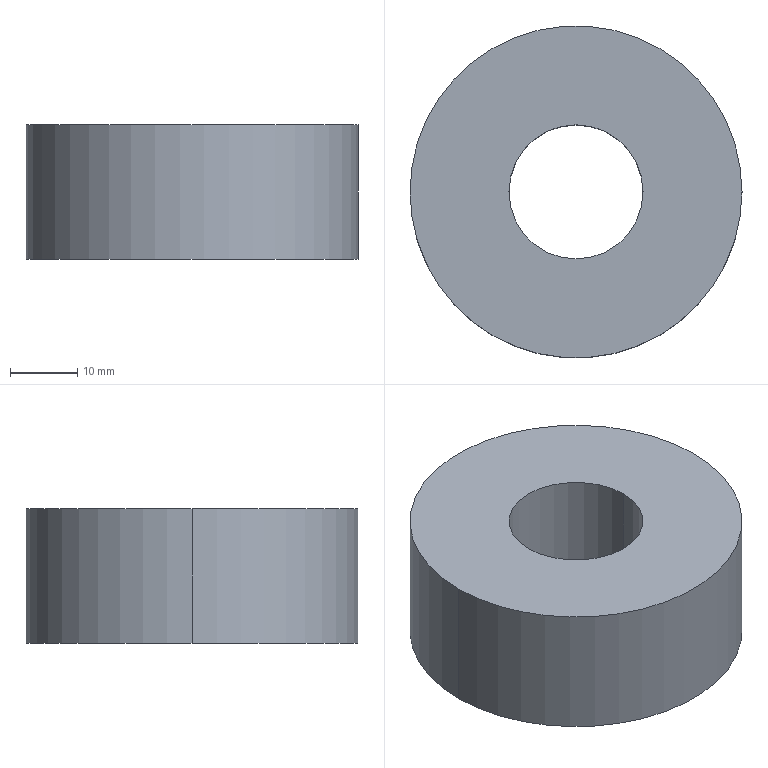Part | SolidWorks | features BaseBody 1 | 1 solid | 6 faces | box 49.497 x 49.497 x 20 mm | volume 32201 mm3 | cylinder 4 | plane 2 | commonest cylinder face diameters 20 x2 49.497 x2
STEP:
#1=CARTESIAN_POINT('',(2518.111,1500.936,20.));
#2=VERTEX_POINT('',#1);
#3=CARTESIAN_POINT('',(2567.609,1500.936,20.));
#4=VERTEX_POINT('',#3);
#5=CARTESIAN_POINT('',(2542.86,1500.936,20.));
#6=DIRECTION('',(0.,0.,-1.));
#7=DIRECTION('',(-1.,0.,0.));
#8=AXIS2_PLACEMENT_3D('',#5,#6,#7);
#9=CIRCLE('',#8,24.749);
#10=EDGE_CURVE('',#2,#4,#9,.T.);
#11=ORIENTED_EDGE('',*,*,#10,.T.);
#12=CARTESIAN_POINT('',(2567.609,1500.936,0.));
#13=VERTEX_POINT('',#12);
#14=CARTESIAN_POINT('',(2567.609,1500.936,20.));
#15=DIRECTION('',(0.,0.,-1.));
#16=VECTOR('',#15,1000.);
#17=LINE('',#14,#16);
#18=EDGE_CURVE('',#4,#13,#17,.T.);
#19=ORIENTED_EDGE('',*,*,#18,.T.);
#20=CARTESIAN_POINT('',(2518.111,1500.936,0.));
#21=VERTEX_POINT('',#20);
#22=CARTESIAN_POINT('',(2542.86,1500.936,0.));
#23=DIRECTION('',(0.,0.,-1.));
#24=DIRECTION('',(-1.,0.,0.));
#25=AXIS2_PLACEMENT_3D('',#22,#23,#24);
#26=CIRCLE('',#25,24.749);
#27=EDGE_CURVE('',#21,#13,#26,.T.);
#28=ORIENTED_EDGE('',*,*,#27,.F.);
#29=CARTESIAN_POINT('',(2518.111,1500.936,20.));
#30=DIRECTION('',(0.,0.,-1.));
#31=VECTOR('',#30,1000.);
#32=LINE('',#29,#31);
#33=EDGE_CURVE('',#2,#21,#32,.T.);
#34=ORIENTED_EDGE('',*,*,#33,.F.);
#35=EDGE_LOOP('',(#11,#19,#28,#34));
#36=FACE_OUTER_BOUND('',#35,.T.);
#37=CARTESIAN_POINT('',(2542.86,1500.936,20.));
#38=DIRECTION('',(0.,0.,-1.));
#39=DIRECTION('',(-1.,0.,0.));
#40=AXIS2_PLACEMENT_3D('',#37,#38,#39);
#41=CYLINDRICAL_SURFACE('',#40,24.749);
#42=ADVANCED_FACE('',(#36),#41,.T.);
#43=CARTESIAN_POINT('',(2552.86,1500.936,20.));
#44=VERTEX_POINT('',#43);
#45=CARTESIAN_POINT('',(2532.86,1500.936,20.));
#46=VERTEX_POINT('',#45);
#47=CARTESIAN_POINT('',(2542.86,1500.936,20.));
#48=DIRECTION('',(0.,0.,-1.));
#49=DIRECTION('',(-1.,0.,0.));
#50=AXIS2_PLACEMENT_3D('',#47,#48,#49);
#51=CIRCLE('',#50,10.);
#52=EDGE_CURVE('',#44,#46,#51,.T.);
#53=ORIENTED_EDGE('',*,*,#52,.F.);
#54=CARTESIAN_POINT('',(2552.86,1500.936,0.));
#55=VERTEX_POINT('',#54);
#56=CARTESIAN_POINT('',(2552.86,1500.936,20.));
#57=DIRECTION('',(0.,0.,-1.));
#58=VECTOR('',#57,1000.);
#59=LINE('',#56,#58);
#60=EDGE_CURVE('',#44,#55,#59,.T.);
#61=ORIENTED_EDGE('',*,*,#60,.T.);
#62=CARTESIAN_POINT('',(2532.86,1500.936,0.));
#63=VERTEX_POINT('',#62);
#64=CARTESIAN_POINT('',(2542.86,1500.936,0.));
#65=DIRECTION('',(0.,0.,-1.));
#66=DIRECTION('',(-1.,0.,0.));
#67=AXIS2_PLACEMENT_3D('',#64,#65,#66);
#68=CIRCLE('',#67,10.);
#69=EDGE_CURVE('',#55,#63,#68,.T.);
#70=ORIENTED_EDGE('',*,*,#69,.T.);
#71=CARTESIAN_POINT('',(2532.86,1500.936,20.));
#72=DIRECTION('',(0.,0.,-1.));
#73=VECTOR('',#72,1000.);
#74=LINE('',#71,#73);
#75=EDGE_CURVE('',#46,#63,#74,.T.);
#76=ORIENTED_EDGE('',*,*,#75,.F.);
#77=EDGE_LOOP('',(#53,#61,#70,#76));
#78=FACE_OUTER_BOUND('',#77,.T.);
#79=CARTESIAN_POINT('',(2542.86,1500.936,20.));
#80=DIRECTION('',(0.,0.,-1.));
#81=DIRECTION('',(-1.,0.,0.));
#82=AXIS2_PLACEMENT_3D('',#79,#80,#81);
#83=CYLINDRICAL_SURFACE('',#82,10.);
#84=ADVANCED_FACE('',(#78),#83,.F.);
#85=ORIENTED_EDGE('',*,*,#60,.F.);
#86=CARTESIAN_POINT('',(2542.86,1500.936,20.));
#87=DIRECTION('',(0.,0.,-1.));
#88=DIRECTION('',(-1.,0.,0.));
#89=AXIS2_PLACEMENT_3D('',#86,#87,#88);
#90=CIRCLE('',#89,10.);
#91=EDGE_CURVE('',#46,#44,#90,.T.);
#92=ORIENTED_EDGE('',*,*,#91,.F.);
#93=ORIENTED_EDGE('',*,*,#75,.T.);
#94=CARTESIAN_POINT('',(2542.86,1500.936,0.));
#95=DIRECTION('',(0.,0.,-1.));
#96=DIRECTION('',(-1.,0.,0.));
#97=AXIS2_PLACEMENT_3D('',#94,#95,#96);
#98=CIRCLE('',#97,10.);
#99=EDGE_CURVE('',#63,#55,#98,.T.);
#100=ORIENTED_EDGE('',*,*,#99,.T.);
#101=EDGE_LOOP('',(#85,#92,#93,#100));
#102=FACE_OUTER_BOUND('',#101,.T.);
#103=CARTESIAN_POINT('',(2542.86,1500.936,20.));
#104=DIRECTION('',(0.,0.,-1.));
#105=DIRECTION('',(-1.,0.,0.));
#106=AXIS2_PLACEMENT_3D('',#103,#104,#105);
#107=CYLINDRICAL_SURFACE('',#106,10.);
#108=ADVANCED_FACE('',(#102),#107,.F.);
#109=ORIENTED_EDGE('',*,*,#27,.T.);
#110=CARTESIAN_POINT('',(2542.86,1500.936,0.));
#111=DIRECTION('',(0.,0.,-1.));
#112=DIRECTION('',(-1.,0.,0.));
#113=AXIS2_PLACEMENT_3D('',#110,#111,#112);
#114=CIRCLE('',#113,24.749);
#115=EDGE_CURVE('',#13,#21,#114,.T.);
#116=ORIENTED_EDGE('',*,*,#115,.T.);
#117=EDGE_LOOP('',(#109,#116));
#118=FACE_OUTER_BOUND('',#117,.T.);
#119=ORIENTED_EDGE('',*,*,#99,.F.);
#120=ORIENTED_EDGE('',*,*,#69,.F.);
#121=EDGE_LOOP('',(#119,#120));
#122=FACE_BOUND('',#121,.T.);
#123=CARTESIAN_POINT('',(2552.86,1500.936,0.));
#124=DIRECTION('',(0.,0.,-1.));
#125=DIRECTION('',(-1.,0.,0.));
#126=AXIS2_PLACEMENT_3D('',#123,#124,#125);
#127=PLANE('',#126);
#128=ADVANCED_FACE('',(#118,#122),#127,.T.);
#129=ORIENTED_EDGE('',*,*,#18,.F.);
#130=CARTESIAN_POINT('',(2542.86,1500.936,20.));
#131=DIRECTION('',(0.,0.,-1.));
#132=DIRECTION('',(-1.,0.,0.));
#133=AXIS2_PLACEMENT_3D('',#130,#131,#132);
#134=CIRCLE('',#133,24.749);
#135=EDGE_CURVE('',#4,#2,#134,.T.);
#136=ORIENTED_EDGE('',*,*,#135,.T.);
#137=ORIENTED_EDGE('',*,*,#33,.T.);
#138=ORIENTED_EDGE('',*,*,#115,.F.);
#139=EDGE_LOOP('',(#129,#136,#137,#138));
#140=FACE_OUTER_BOUND('',#139,.T.);
#141=CARTESIAN_POINT('',(2542.86,1500.936,20.));
#142=DIRECTION('',(0.,0.,-1.));
#143=DIRECTION('',(-1.,0.,0.));
#144=AXIS2_PLACEMENT_3D('',#141,#142,#143);
#145=CYLINDRICAL_SURFACE('',#144,24.749);
#146=ADVANCED_FACE('',(#140),#145,.T.);
#147=ORIENTED_EDGE('',*,*,#91,.T.);
#148=ORIENTED_EDGE('',*,*,#52,.T.);
#149=EDGE_LOOP('',(#147,#148));
#150=FACE_BOUND('',#149,.T.);
#151=ORIENTED_EDGE('',*,*,#10,.F.);
#152=ORIENTED_EDGE('',*,*,#135,.F.);
#153=EDGE_LOOP('',(#151,#152));
#154=FACE_OUTER_BOUND('',#153,.T.);
#155=CARTESIAN_POINT('',(2567.609,1500.936,20.));
#156=DIRECTION('',(0.,0.,1.));
#157=DIRECTION('',(1.,0.,0.));
#158=AXIS2_PLACEMENT_3D('',#155,#156,#157);
#159=PLANE('',#158);
#160=ADVANCED_FACE('',(#150,#154),#159,.T.);
#161=CLOSED_SHELL('',(#42,#84,#108,#128,#146,#160));
#162=MANIFOLD_SOLID_BREP('',#161);
#163=CARTESIAN_POINT('',(0.,0.,0.));
#164=DIRECTION('',(0.,0.,1.));
#165=DIRECTION('',(1.,0.,0.));
#166=AXIS2_PLACEMENT_3D('',#163,#164,#165);
#167=(LENGTH_UNIT()NAMED_UNIT(*)SI_UNIT(.MILLI.,.METRE.));
#168=UNCERTAINTY_MEASURE_WITH_UNIT(LENGTH_MEASURE(0.00001),#167,'','');
#169=(NAMED_UNIT(*)PLANE_ANGLE_UNIT()SI_UNIT($,.RADIAN.));
#170=(NAMED_UNIT(*)SI_UNIT($,.STERADIAN.)SOLID_ANGLE_UNIT());
#171=(GEOMETRIC_REPRESENTATION_CONTEXT(3)GLOBAL_UNCERTAINTY_ASSIGNED_CONTEXT((#168))GLOBAL_UNIT_ASSIGNED_CONTEXT((#167,#169,#170))REPRESENTATION_CONTEXT('',''));
#172=ADVANCED_BREP_SHAPE_REPRESENTATION('',(#162,#166),#171);